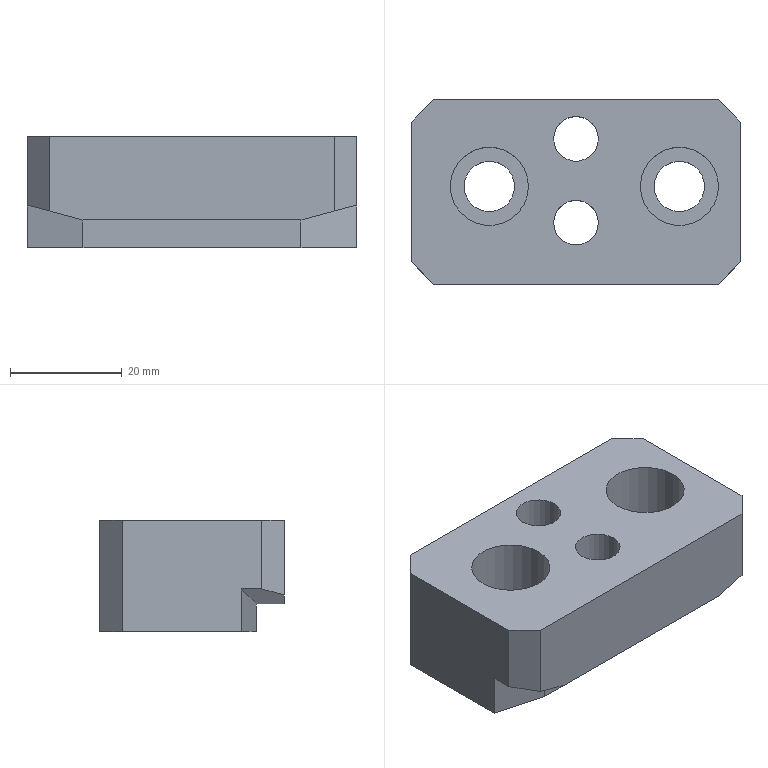Part | NX | features 20 2 | 1 solid | 24 faces | box 59 x 33 x 20 mm | volume 30264 mm3 | plane 18 | cylinder 6 | commonest cylinder face diameters 8.001 x2 9 x2 14 x2
STEP:
#1=CARTESIAN_POINT('',(2760.502,417.5,1.5));
#2=VERTEX_POINT('',#1);
#3=CARTESIAN_POINT('',(2799.502,417.5,1.5));
#4=VERTEX_POINT('',#3);
#5=CARTESIAN_POINT('',(2886.502,417.5,1.5));
#6=DIRECTION('',(1.,0.,0.));
#7=VECTOR('',#6,1000.);
#8=LINE('',#5,#7);
#9=EDGE_CURVE('',#2,#4,#8,.T.);
#10=ORIENTED_EDGE('',*,*,#9,.T.);
#11=CARTESIAN_POINT('',(2805.502,417.5,3.108));
#12=VERTEX_POINT('',#11);
#13=CARTESIAN_POINT('',(2799.502,417.5,1.5));
#14=DIRECTION('',(-0.9659,0.,-0.2588));
#15=VECTOR('',#14,1000.);
#16=LINE('',#13,#15);
#17=EDGE_CURVE('',#12,#4,#16,.T.);
#18=ORIENTED_EDGE('',*,*,#17,.F.);
#19=CARTESIAN_POINT('',(2805.502,417.5,16.5));
#20=VERTEX_POINT('',#19);
#21=CARTESIAN_POINT('',(2805.502,417.5,11.5));
#22=DIRECTION('',(0.,0.,-1.));
#23=VECTOR('',#22,1000.);
#24=LINE('',#21,#23);
#25=EDGE_CURVE('',#20,#12,#24,.T.);
#26=ORIENTED_EDGE('',*,*,#25,.F.);
#27=CARTESIAN_POINT('',(2754.502,417.5,16.5));
#28=VERTEX_POINT('',#27);
#29=CARTESIAN_POINT('',(2908.502,417.5,16.5));
#30=DIRECTION('',(-1.,0.,0.));
#31=VECTOR('',#30,1000.);
#32=LINE('',#29,#31);
#33=EDGE_CURVE('',#20,#28,#32,.T.);
#34=ORIENTED_EDGE('',*,*,#33,.T.);
#35=CARTESIAN_POINT('',(2754.502,417.5,3.108));
#36=VERTEX_POINT('',#35);
#37=CARTESIAN_POINT('',(2754.502,417.5,11.5));
#38=DIRECTION('',(0.,0.,1.));
#39=VECTOR('',#38,1000.);
#40=LINE('',#37,#39);
#41=EDGE_CURVE('',#36,#28,#40,.T.);
#42=ORIENTED_EDGE('',*,*,#41,.F.);
#43=CARTESIAN_POINT('',(2760.502,417.5,1.5));
#44=DIRECTION('',(-0.9659,0.,0.2588));
#45=VECTOR('',#44,1000.);
#46=LINE('',#43,#45);
#47=EDGE_CURVE('',#2,#36,#46,.T.);
#48=ORIENTED_EDGE('',*,*,#47,.F.);
#49=EDGE_LOOP('',(#10,#18,#26,#34,#42,#48));
#50=FACE_BOUND('',#49,.T.);
#51=CARTESIAN_POINT('',(2908.502,417.5,11.5));
#52=DIRECTION('',(0.,1.,0.));
#53=DIRECTION('',(0.,0.,1.));
#54=AXIS2_PLACEMENT_3D('',#51,#52,#53);
#55=PLANE('',#54);
#56=ADVANCED_FACE('',(#50),#55,.F.);
#57=CARTESIAN_POINT('',(2784.003,428.5,16.5));
#58=VERTEX_POINT('',#57);
#59=CARTESIAN_POINT('',(2780.002,428.5,16.5));
#60=DIRECTION('',(0.,0.,1.));
#61=DIRECTION('',(1.,0.,0.));
#62=AXIS2_PLACEMENT_3D('',#59,#60,#61);
#63=CIRCLE('',#62,4.);
#64=EDGE_CURVE('',#58,#58,#63,.T.);
#65=ORIENTED_EDGE('',*,*,#64,.F.);
#66=EDGE_LOOP('',(#65));
#67=FACE_BOUND('',#66,.T.);
#68=CARTESIAN_POINT('',(2784.003,443.5,16.5));
#69=VERTEX_POINT('',#68);
#70=CARTESIAN_POINT('',(2780.002,443.5,16.5));
#71=DIRECTION('',(0.,0.,1.));
#72=DIRECTION('',(1.,0.,0.));
#73=AXIS2_PLACEMENT_3D('',#70,#71,#72);
#74=CIRCLE('',#73,4.);
#75=EDGE_CURVE('',#69,#69,#74,.T.);
#76=ORIENTED_EDGE('',*,*,#75,.F.);
#77=EDGE_LOOP('',(#76));
#78=FACE_BOUND('',#77,.T.);
#79=CARTESIAN_POINT('',(2805.502,435.,16.5));
#80=VERTEX_POINT('',#79);
#81=CARTESIAN_POINT('',(2798.502,435.,16.5));
#82=DIRECTION('',(0.,0.,-1.));
#83=DIRECTION('',(1.,0.,0.));
#84=AXIS2_PLACEMENT_3D('',#81,#82,#83);
#85=CIRCLE('',#84,7.);
#86=EDGE_CURVE('',#80,#80,#85,.T.);
#87=ORIENTED_EDGE('',*,*,#86,.T.);
#88=EDGE_LOOP('',(#87));
#89=FACE_BOUND('',#88,.T.);
#90=CARTESIAN_POINT('',(2771.502,435.,16.5));
#91=VERTEX_POINT('',#90);
#92=CARTESIAN_POINT('',(2764.502,435.,16.5));
#93=DIRECTION('',(0.,0.,-1.));
#94=DIRECTION('',(1.,0.,0.));
#95=AXIS2_PLACEMENT_3D('',#92,#93,#94);
#96=CIRCLE('',#95,7.);
#97=EDGE_CURVE('',#91,#91,#96,.T.);
#98=ORIENTED_EDGE('',*,*,#97,.T.);
#99=EDGE_LOOP('',(#98));
#100=FACE_BOUND('',#99,.T.);
#101=ORIENTED_EDGE('',*,*,#33,.F.);
#102=CARTESIAN_POINT('',(2809.502,421.5,16.5));
#103=VERTEX_POINT('',#102);
#104=CARTESIAN_POINT('',(2805.502,417.5,16.5));
#105=DIRECTION('',(-0.7071,-0.7071,0.));
#106=VECTOR('',#105,1000.);
#107=LINE('',#104,#106);
#108=EDGE_CURVE('',#103,#20,#107,.T.);
#109=ORIENTED_EDGE('',*,*,#108,.F.);
#110=CARTESIAN_POINT('',(2809.502,446.5,16.5));
#111=VERTEX_POINT('',#110);
#112=CARTESIAN_POINT('',(2809.502,450.5,16.5));
#113=DIRECTION('',(0.,-1.,0.));
#114=VECTOR('',#113,1000.);
#115=LINE('',#112,#114);
#116=EDGE_CURVE('',#111,#103,#115,.T.);
#117=ORIENTED_EDGE('',*,*,#116,.F.);
#118=CARTESIAN_POINT('',(2805.502,450.5,16.5));
#119=VERTEX_POINT('',#118);
#120=CARTESIAN_POINT('',(2809.502,446.5,16.5));
#121=DIRECTION('',(0.7071,-0.7071,0.));
#122=VECTOR('',#121,1000.);
#123=LINE('',#120,#122);
#124=EDGE_CURVE('',#119,#111,#123,.T.);
#125=ORIENTED_EDGE('',*,*,#124,.F.);
#126=CARTESIAN_POINT('',(2754.502,450.5,16.5));
#127=VERTEX_POINT('',#126);
#128=CARTESIAN_POINT('',(2828.502,450.5,16.5));
#129=DIRECTION('',(1.,0.,0.));
#130=VECTOR('',#129,1000.);
#131=LINE('',#128,#130);
#132=EDGE_CURVE('',#127,#119,#131,.T.);
#133=ORIENTED_EDGE('',*,*,#132,.F.);
#134=CARTESIAN_POINT('',(2750.502,446.5,16.5));
#135=VERTEX_POINT('',#134);
#136=CARTESIAN_POINT('',(2754.502,450.5,16.5));
#137=DIRECTION('',(0.7071,0.7071,0.));
#138=VECTOR('',#137,1000.);
#139=LINE('',#136,#138);
#140=EDGE_CURVE('',#135,#127,#139,.T.);
#141=ORIENTED_EDGE('',*,*,#140,.F.);
#142=CARTESIAN_POINT('',(2750.502,421.5,16.5));
#143=VERTEX_POINT('',#142);
#144=CARTESIAN_POINT('',(2750.502,417.5,16.5));
#145=DIRECTION('',(0.,1.,0.));
#146=VECTOR('',#145,1000.);
#147=LINE('',#144,#146);
#148=EDGE_CURVE('',#143,#135,#147,.T.);
#149=ORIENTED_EDGE('',*,*,#148,.F.);
#150=CARTESIAN_POINT('',(2750.502,421.5,16.5));
#151=DIRECTION('',(-0.7071,0.7071,0.));
#152=VECTOR('',#151,1000.);
#153=LINE('',#150,#152);
#154=EDGE_CURVE('',#28,#143,#153,.T.);
#155=ORIENTED_EDGE('',*,*,#154,.F.);
#156=EDGE_LOOP('',(#101,#109,#117,#125,#133,#141,#149,#155));
#157=FACE_BOUND('',#156,.T.);
#158=CARTESIAN_POINT('',(2908.502,450.5,16.5));
#159=DIRECTION('',(0.,0.,1.));
#160=DIRECTION('',(-1.,0.,0.));
#161=AXIS2_PLACEMENT_3D('',#158,#159,#160);
#162=PLANE('',#161);
#163=ADVANCED_FACE('',(#67,#78,#89,#100,#157),#162,.T.);
#164=CARTESIAN_POINT('',(2794.002,435.,6.5));
#165=VERTEX_POINT('',#164);
#166=CARTESIAN_POINT('',(2798.502,435.,6.5));
#167=DIRECTION('',(0.,0.,1.));
#168=DIRECTION('',(-1.,0.,0.));
#169=AXIS2_PLACEMENT_3D('',#166,#167,#168);
#170=CIRCLE('',#169,4.5);
#171=EDGE_CURVE('',#165,#165,#170,.T.);
#172=ORIENTED_EDGE('',*,*,#171,.F.);
#173=EDGE_LOOP('',(#172));
#174=FACE_BOUND('',#173,.T.);
#175=CARTESIAN_POINT('',(2791.502,435.,6.5));
#176=VERTEX_POINT('',#175);
#177=CARTESIAN_POINT('',(2798.502,435.,6.5));
#178=DIRECTION('',(0.,0.,-1.));
#179=DIRECTION('',(-1.,0.,0.));
#180=AXIS2_PLACEMENT_3D('',#177,#178,#179);
#181=CIRCLE('',#180,7.);
#182=EDGE_CURVE('',#176,#176,#181,.T.);
#183=ORIENTED_EDGE('',*,*,#182,.F.);
#184=EDGE_LOOP('',(#183));
#185=FACE_BOUND('',#184,.T.);
#186=CARTESIAN_POINT('',(2798.502,432.5,6.5));
#187=DIRECTION('',(0.,0.,-1.));
#188=DIRECTION('',(1.,0.,0.));
#189=AXIS2_PLACEMENT_3D('',#186,#187,#188);
#190=PLANE('',#189);
#191=ADVANCED_FACE('',(#174,#185),#190,.F.);
#192=CARTESIAN_POINT('',(2799.502,422.5,1.5));
#193=VERTEX_POINT('',#192);
#194=CARTESIAN_POINT('',(2799.502,425.18,1.5));
#195=DIRECTION('',(0.,1.,0.));
#196=VECTOR('',#195,1000.);
#197=LINE('',#194,#196);
#198=EDGE_CURVE('',#4,#193,#197,.T.);
#199=ORIENTED_EDGE('',*,*,#198,.T.);
#200=CARTESIAN_POINT('',(2809.502,425.18,4.179));
#201=VERTEX_POINT('',#200);
#202=CARTESIAN_POINT('',(2808.875,425.012,4.011));
#203=DIRECTION('',(0.9351,0.2506,0.2506));
#204=VECTOR('',#203,1000.);
#205=LINE('',#202,#204);
#206=EDGE_CURVE('',#193,#201,#205,.T.);
#207=ORIENTED_EDGE('',*,*,#206,.T.);
#208=CARTESIAN_POINT('',(2809.502,421.5,4.179));
#209=VERTEX_POINT('',#208);
#210=CARTESIAN_POINT('',(2809.502,417.5,4.179));
#211=DIRECTION('',(0.,-1.,0.));
#212=VECTOR('',#211,1000.);
#213=LINE('',#210,#212);
#214=EDGE_CURVE('',#201,#209,#213,.T.);
#215=ORIENTED_EDGE('',*,*,#214,.T.);
#216=CARTESIAN_POINT('',(2792.451,404.449,-0.3894));
#217=DIRECTION('',(0.6947,0.6947,0.1862));
#218=VECTOR('',#217,1000.);
#219=LINE('',#216,#218);
#220=EDGE_CURVE('',#12,#209,#219,.T.);
#221=ORIENTED_EDGE('',*,*,#220,.F.);
#222=ORIENTED_EDGE('',*,*,#17,.T.);
#223=EDGE_LOOP('',(#199,#207,#215,#221,#222));
#224=FACE_BOUND('',#223,.T.);
#225=CARTESIAN_POINT('',(2799.502,396.891,1.5));
#226=DIRECTION('',(0.2588,0.,-0.9659));
#227=DIRECTION('',(0.9659,0.,0.2588));
#228=AXIS2_PLACEMENT_3D('',#225,#226,#227);
#229=PLANE('',#228);
#230=ADVANCED_FACE('',(#224),#229,.T.);
#231=CARTESIAN_POINT('',(2760.002,435.,6.5));
#232=VERTEX_POINT('',#231);
#233=CARTESIAN_POINT('',(2764.502,435.,6.5));
#234=DIRECTION('',(0.,0.,1.));
#235=DIRECTION('',(-1.,0.,0.));
#236=AXIS2_PLACEMENT_3D('',#233,#234,#235);
#237=CIRCLE('',#236,4.5);
#238=EDGE_CURVE('',#232,#232,#237,.T.);
#239=ORIENTED_EDGE('',*,*,#238,.F.);
#240=EDGE_LOOP('',(#239));
#241=FACE_BOUND('',#240,.T.);
#242=CARTESIAN_POINT('',(2757.502,435.,6.5));
#243=VERTEX_POINT('',#242);
#244=CARTESIAN_POINT('',(2764.502,435.,6.5));
#245=DIRECTION('',(0.,0.,-1.));
#246=DIRECTION('',(-1.,0.,0.));
#247=AXIS2_PLACEMENT_3D('',#244,#245,#246);
#248=CIRCLE('',#247,7.);
#249=EDGE_CURVE('',#243,#243,#248,.T.);
#250=ORIENTED_EDGE('',*,*,#249,.F.);
#251=EDGE_LOOP('',(#250));
#252=FACE_BOUND('',#251,.T.);
#253=CARTESIAN_POINT('',(2764.502,432.5,6.5));
#254=DIRECTION('',(0.,0.,-1.));
#255=DIRECTION('',(-1.,0.,0.));
#256=AXIS2_PLACEMENT_3D('',#253,#254,#255);
#257=PLANE('',#256);
#258=ADVANCED_FACE('',(#241,#252),#257,.F.);
#259=ORIENTED_EDGE('',*,*,#86,.F.);
#260=EDGE_LOOP('',(#259));
#261=FACE_BOUND('',#260,.T.);
#262=ORIENTED_EDGE('',*,*,#182,.T.);
#263=EDGE_LOOP('',(#262));
#264=FACE_BOUND('',#263,.T.);
#265=CARTESIAN_POINT('',(2798.502,435.,42.5));
#266=DIRECTION('',(0.,0.,-1.));
#267=DIRECTION('',(1.,0.,0.));
#268=AXIS2_PLACEMENT_3D('',#265,#266,#267);
#269=CYLINDRICAL_SURFACE('',#268,7.);
#270=ADVANCED_FACE('',(#261,#264),#269,.F.);
#271=ORIENTED_EDGE('',*,*,#108,.T.);
#272=ORIENTED_EDGE('',*,*,#25,.T.);
#273=ORIENTED_EDGE('',*,*,#220,.T.);
#274=CARTESIAN_POINT('',(2809.502,421.5,11.5));
#275=DIRECTION('',(0.,0.,1.));
#276=VECTOR('',#275,1000.);
#277=LINE('',#274,#276);
#278=EDGE_CURVE('',#209,#103,#277,.T.);
#279=ORIENTED_EDGE('',*,*,#278,.T.);
#280=EDGE_LOOP('',(#271,#272,#273,#279));
#281=FACE_BOUND('',#280,.T.);
#282=CARTESIAN_POINT('',(2805.502,417.5,11.5));
#283=DIRECTION('',(-0.7071,0.7071,0.));
#284=DIRECTION('',(0.,0.,-1.));
#285=AXIS2_PLACEMENT_3D('',#282,#283,#284);
#286=PLANE('',#285);
#287=ADVANCED_FACE('',(#281),#286,.F.);
#288=ORIENTED_EDGE('',*,*,#249,.T.);
#289=EDGE_LOOP('',(#288));
#290=FACE_BOUND('',#289,.T.);
#291=ORIENTED_EDGE('',*,*,#97,.F.);
#292=EDGE_LOOP('',(#291));
#293=FACE_BOUND('',#292,.T.);
#294=CARTESIAN_POINT('',(2764.502,435.,42.5));
#295=DIRECTION('',(0.,0.,-1.));
#296=DIRECTION('',(-1.,0.,0.));
#297=AXIS2_PLACEMENT_3D('',#294,#295,#296);
#298=CYLINDRICAL_SURFACE('',#297,7.);
#299=ADVANCED_FACE('',(#290,#293),#298,.F.);
#300=ORIENTED_EDGE('',*,*,#214,.F.);
#301=CARTESIAN_POINT('',(2809.502,425.18,-3.5));
#302=VERTEX_POINT('',#301);
#303=CARTESIAN_POINT('',(2809.502,425.18,3.5));
#304=DIRECTION('',(0.,0.,-1.));
#305=VECTOR('',#304,1000.);
#306=LINE('',#303,#305);
#307=EDGE_CURVE('',#201,#302,#306,.T.);
#308=ORIENTED_EDGE('',*,*,#307,.T.);
#309=CARTESIAN_POINT('',(2809.502,446.5,-3.5));
#310=VERTEX_POINT('',#309);
#311=CARTESIAN_POINT('',(2809.502,450.5,-3.5));
#312=DIRECTION('',(0.,-1.,0.));
#313=VECTOR('',#312,1000.);
#314=LINE('',#311,#313);
#315=EDGE_CURVE('',#310,#302,#314,.T.);
#316=ORIENTED_EDGE('',*,*,#315,.F.);
#317=CARTESIAN_POINT('',(2809.502,446.5,11.5));
#318=DIRECTION('',(0.,0.,-1.));
#319=VECTOR('',#318,1000.);
#320=LINE('',#317,#319);
#321=EDGE_CURVE('',#111,#310,#320,.T.);
#322=ORIENTED_EDGE('',*,*,#321,.F.);
#323=ORIENTED_EDGE('',*,*,#116,.T.);
#324=ORIENTED_EDGE('',*,*,#278,.F.);
#325=EDGE_LOOP('',(#300,#308,#316,#322,#323,#324));
#326=FACE_BOUND('',#325,.T.);
#327=CARTESIAN_POINT('',(2809.502,450.5,11.5));
#328=DIRECTION('',(-1.,0.,0.));
#329=DIRECTION('',(0.,0.,-1.));
#330=AXIS2_PLACEMENT_3D('',#327,#328,#329);
#331=PLANE('',#330);
#332=ADVANCED_FACE('',(#326),#331,.F.);
#333=CARTESIAN_POINT('',(2799.501,422.5,1.5));
#334=VERTEX_POINT('',#333);
#335=CARTESIAN_POINT('',(2809.502,425.18,1.5));
#336=DIRECTION('',(0.9659,0.2588,0.));
#337=VECTOR('',#336,1000.);
#338=LINE('',#335,#337);
#339=EDGE_CURVE('',#334,#193,#338,.T.);
#340=ORIENTED_EDGE('',*,*,#339,.F.);
#341=CARTESIAN_POINT('',(2799.501,422.5,-3.5));
#342=VERTEX_POINT('',#341);
#343=CARTESIAN_POINT('',(2799.501,422.5,3.5));
#344=DIRECTION('',(0.,0.,1.));
#345=VECTOR('',#344,1000.);
#346=LINE('',#343,#345);
#347=EDGE_CURVE('',#342,#334,#346,.T.);
#348=ORIENTED_EDGE('',*,*,#347,.F.);
#349=CARTESIAN_POINT('',(2809.502,425.18,-3.5));
#350=DIRECTION('',(-0.9659,-0.2588,0.));
#351=VECTOR('',#350,1000.);
#352=LINE('',#349,#351);
#353=EDGE_CURVE('',#302,#342,#352,.T.);
#354=ORIENTED_EDGE('',*,*,#353,.F.);
#355=ORIENTED_EDGE('',*,*,#307,.F.);
#356=ORIENTED_EDGE('',*,*,#206,.F.);
#357=EDGE_LOOP('',(#340,#348,#354,#355,#356));
#358=FACE_BOUND('',#357,.T.);
#359=CARTESIAN_POINT('',(2809.502,425.18,3.5));
#360=DIRECTION('',(-0.2588,0.9659,0.));
#361=DIRECTION('',(0.9659,0.2588,0.));
#362=AXIS2_PLACEMENT_3D('',#359,#360,#361);
#363=PLANE('',#362);
#364=ADVANCED_FACE('',(#358),#363,.F.);
#365=ORIENTED_EDGE('',*,*,#171,.T.);
#366=EDGE_LOOP('',(#365));
#367=FACE_BOUND('',#366,.T.);
#368=CARTESIAN_POINT('',(2803.002,435.,-3.5));
#369=VERTEX_POINT('',#368);
#370=CARTESIAN_POINT('',(2798.502,435.,-3.5));
#371=DIRECTION('',(0.,0.,-1.));
#372=DIRECTION('',(1.,0.,0.));
#373=AXIS2_PLACEMENT_3D('',#370,#371,#372);
#374=CIRCLE('',#373,4.5);
#375=EDGE_CURVE('',#369,#369,#374,.T.);
#376=ORIENTED_EDGE('',*,*,#375,.T.);
#377=EDGE_LOOP('',(#376));
#378=FACE_BOUND('',#377,.T.);
#379=CARTESIAN_POINT('',(2798.502,435.,42.5));
#380=DIRECTION('',(0.,0.,-1.));
#381=DIRECTION('',(1.,0.,0.));
#382=AXIS2_PLACEMENT_3D('',#379,#380,#381);
#383=CYLINDRICAL_SURFACE('',#382,4.5);
#384=ADVANCED_FACE('',(#367,#378),#383,.F.);
#385=CARTESIAN_POINT('',(2750.502,421.5,4.179));
#386=VERTEX_POINT('',#385);
#387=CARTESIAN_POINT('',(2750.502,421.5,11.5));
#388=DIRECTION('',(0.,0.,-1.));
#389=VECTOR('',#388,1000.);
#390=LINE('',#387,#389);
#391=EDGE_CURVE('',#143,#386,#390,.T.);
#392=ORIENTED_EDGE('',*,*,#391,.T.);
#393=CARTESIAN_POINT('',(2767.554,404.449,-0.3894));
#394=DIRECTION('',(0.6947,-0.6947,-0.1862));
#395=VECTOR('',#394,1000.);
#396=LINE('',#393,#395);
#397=EDGE_CURVE('',#386,#36,#396,.T.);
#398=ORIENTED_EDGE('',*,*,#397,.T.);
#399=ORIENTED_EDGE('',*,*,#41,.T.);
#400=ORIENTED_EDGE('',*,*,#154,.T.);
#401=EDGE_LOOP('',(#392,#398,#399,#400));
#402=FACE_BOUND('',#401,.T.);
#403=CARTESIAN_POINT('',(2750.502,421.5,11.5));
#404=DIRECTION('',(0.7071,0.7071,0.));
#405=DIRECTION('',(0.,0.,-1.));
#406=AXIS2_PLACEMENT_3D('',#403,#404,#405);
#407=PLANE('',#406);
#408=ADVANCED_FACE('',(#402),#407,.F.);
#409=CARTESIAN_POINT('',(2769.002,435.,-3.5));
#410=VERTEX_POINT('',#409);
#411=CARTESIAN_POINT('',(2764.502,435.,-3.5));
#412=DIRECTION('',(0.,0.,1.));
#413=DIRECTION('',(1.,0.,0.));
#414=AXIS2_PLACEMENT_3D('',#411,#412,#413);
#415=CIRCLE('',#414,4.5);
#416=EDGE_CURVE('',#410,#410,#415,.T.);
#417=ORIENTED_EDGE('',*,*,#416,.F.);
#418=EDGE_LOOP('',(#417));
#419=FACE_BOUND('',#418,.T.);
#420=ORIENTED_EDGE('',*,*,#238,.T.);
#421=EDGE_LOOP('',(#420));
#422=FACE_BOUND('',#421,.T.);
#423=CARTESIAN_POINT('',(2764.502,435.,42.5));
#424=DIRECTION('',(0.,0.,-1.));
#425=DIRECTION('',(-1.,0.,0.));
#426=AXIS2_PLACEMENT_3D('',#423,#424,#425);
#427=CYLINDRICAL_SURFACE('',#426,4.5);
#428=ADVANCED_FACE('',(#419,#422),#427,.F.);
#429=CARTESIAN_POINT('',(2750.502,425.179,-3.5));
#430=VERTEX_POINT('',#429);
#431=CARTESIAN_POINT('',(2750.502,446.5,-3.5));
#432=VERTEX_POINT('',#431);
#433=CARTESIAN_POINT('',(2750.502,417.5,-3.5));
#434=DIRECTION('',(0.,1.,0.));
#435=VECTOR('',#434,1000.);
#436=LINE('',#433,#435);
#437=EDGE_CURVE('',#430,#432,#436,.T.);
#438=ORIENTED_EDGE('',*,*,#437,.F.);
#439=CARTESIAN_POINT('',(2750.502,425.179,4.179));
#440=VERTEX_POINT('',#439);
#441=CARTESIAN_POINT('',(2750.502,425.179,3.5));
#442=DIRECTION('',(0.,0.,-1.));
#443=VECTOR('',#442,1000.);
#444=LINE('',#441,#443);
#445=EDGE_CURVE('',#440,#430,#444,.T.);
#446=ORIENTED_EDGE('',*,*,#445,.F.);
#447=CARTESIAN_POINT('',(2750.502,425.179,4.179));
#448=DIRECTION('',(0.,1.,0.));
#449=VECTOR('',#448,1000.);
#450=LINE('',#447,#449);
#451=EDGE_CURVE('',#386,#440,#450,.T.);
#452=ORIENTED_EDGE('',*,*,#451,.F.);
#453=ORIENTED_EDGE('',*,*,#391,.F.);
#454=ORIENTED_EDGE('',*,*,#148,.T.);
#455=CARTESIAN_POINT('',(2750.502,446.5,11.5));
#456=DIRECTION('',(0.,0.,1.));
#457=VECTOR('',#456,1000.);
#458=LINE('',#455,#457);
#459=EDGE_CURVE('',#432,#135,#458,.T.);
#460=ORIENTED_EDGE('',*,*,#459,.F.);
#461=EDGE_LOOP('',(#438,#446,#452,#453,#454,#460));
#462=FACE_BOUND('',#461,.T.);
#463=CARTESIAN_POINT('',(2750.502,417.5,11.5));
#464=DIRECTION('',(1.,0.,0.));
#465=DIRECTION('',(0.,0.,1.));
#466=AXIS2_PLACEMENT_3D('',#463,#464,#465);
#467=PLANE('',#466);
#468=ADVANCED_FACE('',(#462),#467,.F.);
#469=ORIENTED_EDGE('',*,*,#451,.T.);
#470=CARTESIAN_POINT('',(2760.501,422.5,1.5));
#471=VERTEX_POINT('',#470);
#472=CARTESIAN_POINT('',(2760.501,422.5,1.5));
#473=DIRECTION('',(0.9351,-0.2506,-0.2506));
#474=VECTOR('',#473,1000.);
#475=LINE('',#472,#474);
#476=EDGE_CURVE('',#440,#471,#475,.T.);
#477=ORIENTED_EDGE('',*,*,#476,.T.);
#478=CARTESIAN_POINT('',(2760.502,422.5,1.5));
#479=VERTEX_POINT('',#478);
#480=CARTESIAN_POINT('',(2760.502,422.5,1.5));
#481=DIRECTION('',(0.9659,0.,-0.2588));
#482=VECTOR('',#481,1000.);
#483=LINE('',#480,#482);
#484=EDGE_CURVE('',#471,#479,#483,.T.);
#485=ORIENTED_EDGE('',*,*,#484,.T.);
#486=CARTESIAN_POINT('',(2760.502,417.5,1.5));
#487=DIRECTION('',(0.,-1.,0.));
#488=VECTOR('',#487,1000.);
#489=LINE('',#486,#488);
#490=EDGE_CURVE('',#479,#2,#489,.T.);
#491=ORIENTED_EDGE('',*,*,#490,.T.);
#492=ORIENTED_EDGE('',*,*,#47,.T.);
#493=ORIENTED_EDGE('',*,*,#397,.F.);
#494=EDGE_LOOP('',(#469,#477,#485,#491,#492,#493));
#495=FACE_BOUND('',#494,.T.);
#496=CARTESIAN_POINT('',(2760.502,396.891,1.5));
#497=DIRECTION('',(-0.2588,0.,-0.9659));
#498=DIRECTION('',(0.9659,0.,-0.2588));
#499=AXIS2_PLACEMENT_3D('',#496,#497,#498);
#500=PLANE('',#499);
#501=ADVANCED_FACE('',(#495),#500,.T.);
#502=CARTESIAN_POINT('',(2760.501,422.5,-3.5));
#503=VERTEX_POINT('',#502);
#504=CARTESIAN_POINT('',(2760.501,422.5,-3.5));
#505=DIRECTION('',(-0.9659,0.2588,0.));
#506=VECTOR('',#505,1000.);
#507=LINE('',#504,#506);
#508=EDGE_CURVE('',#503,#430,#507,.T.);
#509=ORIENTED_EDGE('',*,*,#508,.F.);
#510=CARTESIAN_POINT('',(2760.501,422.5,3.5));
#511=DIRECTION('',(0.,0.,1.));
#512=VECTOR('',#511,1000.);
#513=LINE('',#510,#512);
#514=EDGE_CURVE('',#503,#471,#513,.T.);
#515=ORIENTED_EDGE('',*,*,#514,.T.);
#516=ORIENTED_EDGE('',*,*,#476,.F.);
#517=ORIENTED_EDGE('',*,*,#445,.T.);
#518=EDGE_LOOP('',(#509,#515,#516,#517));
#519=FACE_BOUND('',#518,.T.);
#520=CARTESIAN_POINT('',(2760.501,422.5,3.5));
#521=DIRECTION('',(0.2588,0.9659,0.));
#522=DIRECTION('',(0.9659,-0.2588,0.));
#523=AXIS2_PLACEMENT_3D('',#520,#521,#522);
#524=PLANE('',#523);
#525=ADVANCED_FACE('',(#519),#524,.F.);
#526=CARTESIAN_POINT('',(2784.003,428.5,-3.5));
#527=VERTEX_POINT('',#526);
#528=CARTESIAN_POINT('',(2780.002,428.5,-3.5));
#529=DIRECTION('',(0.,0.,1.));
#530=DIRECTION('',(1.,0.,0.));
#531=AXIS2_PLACEMENT_3D('',#528,#529,#530);
#532=CIRCLE('',#531,4.);
#533=EDGE_CURVE('',#527,#527,#532,.T.);
#534=ORIENTED_EDGE('',*,*,#533,.T.);
#535=EDGE_LOOP('',(#534));
#536=FACE_BOUND('',#535,.T.);
#537=CARTESIAN_POINT('',(2784.003,443.5,-3.5));
#538=VERTEX_POINT('',#537);
#539=CARTESIAN_POINT('',(2780.002,443.5,-3.5));
#540=DIRECTION('',(0.,0.,1.));
#541=DIRECTION('',(1.,0.,0.));
#542=AXIS2_PLACEMENT_3D('',#539,#540,#541);
#543=CIRCLE('',#542,4.);
#544=EDGE_CURVE('',#538,#538,#543,.T.);
#545=ORIENTED_EDGE('',*,*,#544,.T.);
#546=EDGE_LOOP('',(#545));
#547=FACE_BOUND('',#546,.T.);
#548=CARTESIAN_POINT('',(2846.501,422.5,-3.5));
#549=DIRECTION('',(-1.,0.,0.));
#550=VECTOR('',#549,1000.);
#551=LINE('',#548,#550);
#552=EDGE_CURVE('',#342,#503,#551,.T.);
#553=ORIENTED_EDGE('',*,*,#552,.T.);
#554=ORIENTED_EDGE('',*,*,#508,.T.);
#555=ORIENTED_EDGE('',*,*,#437,.T.);
#556=CARTESIAN_POINT('',(2754.502,450.5,-3.5));
#557=VERTEX_POINT('',#556);
#558=CARTESIAN_POINT('',(2754.502,450.5,-3.5));
#559=DIRECTION('',(-0.7071,-0.7071,0.));
#560=VECTOR('',#559,1000.);
#561=LINE('',#558,#560);
#562=EDGE_CURVE('',#557,#432,#561,.T.);
#563=ORIENTED_EDGE('',*,*,#562,.F.);
#564=CARTESIAN_POINT('',(2805.502,450.5,-3.5));
#565=VERTEX_POINT('',#564);
#566=CARTESIAN_POINT('',(2868.502,450.5,-3.5));
#567=DIRECTION('',(1.,0.,0.));
#568=VECTOR('',#567,1000.);
#569=LINE('',#566,#568);
#570=EDGE_CURVE('',#557,#565,#569,.T.);
#571=ORIENTED_EDGE('',*,*,#570,.T.);
#572=CARTESIAN_POINT('',(2809.502,446.5,-3.5));
#573=DIRECTION('',(-0.7071,0.7071,0.));
#574=VECTOR('',#573,1000.);
#575=LINE('',#572,#574);
#576=EDGE_CURVE('',#310,#565,#575,.T.);
#577=ORIENTED_EDGE('',*,*,#576,.F.);
#578=ORIENTED_EDGE('',*,*,#315,.T.);
#579=ORIENTED_EDGE('',*,*,#353,.T.);
#580=EDGE_LOOP('',(#553,#554,#555,#563,#571,#577,#578,#579));
#581=FACE_BOUND('',#580,.T.);
#582=ORIENTED_EDGE('',*,*,#416,.T.);
#583=EDGE_LOOP('',(#582));
#584=FACE_BOUND('',#583,.T.);
#585=ORIENTED_EDGE('',*,*,#375,.F.);
#586=EDGE_LOOP('',(#585));
#587=FACE_BOUND('',#586,.T.);
#588=CARTESIAN_POINT('',(2938.502,450.5,-3.5));
#589=DIRECTION('',(0.,0.,1.));
#590=DIRECTION('',(-1.,0.,0.));
#591=AXIS2_PLACEMENT_3D('',#588,#589,#590);
#592=PLANE('',#591);
#593=ADVANCED_FACE('',(#536,#547,#581,#584,#587),#592,.F.);
#594=ORIENTED_EDGE('',*,*,#562,.T.);
#595=ORIENTED_EDGE('',*,*,#459,.T.);
#596=ORIENTED_EDGE('',*,*,#140,.T.);
#597=CARTESIAN_POINT('',(2754.502,450.5,11.5));
#598=DIRECTION('',(0.,0.,-1.));
#599=VECTOR('',#598,1000.);
#600=LINE('',#597,#599);
#601=EDGE_CURVE('',#127,#557,#600,.T.);
#602=ORIENTED_EDGE('',*,*,#601,.T.);
#603=EDGE_LOOP('',(#594,#595,#596,#602));
#604=FACE_BOUND('',#603,.T.);
#605=CARTESIAN_POINT('',(2754.502,450.5,11.5));
#606=DIRECTION('',(0.7071,-0.7071,0.));
#607=DIRECTION('',(0.,0.,-1.));
#608=AXIS2_PLACEMENT_3D('',#605,#606,#607);
#609=PLANE('',#608);
#610=ADVANCED_FACE('',(#604),#609,.F.);
#611=ORIENTED_EDGE('',*,*,#576,.T.);
#612=CARTESIAN_POINT('',(2805.502,450.5,11.5));
#613=DIRECTION('',(0.,0.,1.));
#614=VECTOR('',#613,1000.);
#615=LINE('',#612,#614);
#616=EDGE_CURVE('',#565,#119,#615,.T.);
#617=ORIENTED_EDGE('',*,*,#616,.T.);
#618=ORIENTED_EDGE('',*,*,#124,.T.);
#619=ORIENTED_EDGE('',*,*,#321,.T.);
#620=EDGE_LOOP('',(#611,#617,#618,#619));
#621=FACE_BOUND('',#620,.T.);
#622=CARTESIAN_POINT('',(2809.502,446.5,11.5));
#623=DIRECTION('',(-0.7071,-0.7071,0.));
#624=DIRECTION('',(0.,0.,-1.));
#625=AXIS2_PLACEMENT_3D('',#622,#623,#624);
#626=PLANE('',#625);
#627=ADVANCED_FACE('',(#621),#626,.F.);
#628=ORIENTED_EDGE('',*,*,#616,.F.);
#629=ORIENTED_EDGE('',*,*,#570,.F.);
#630=ORIENTED_EDGE('',*,*,#601,.F.);
#631=ORIENTED_EDGE('',*,*,#132,.T.);
#632=EDGE_LOOP('',(#628,#629,#630,#631));
#633=FACE_BOUND('',#632,.T.);
#634=CARTESIAN_POINT('',(2828.502,450.5,11.5));
#635=DIRECTION('',(0.,-1.,0.));
#636=DIRECTION('',(0.,0.,-1.));
#637=AXIS2_PLACEMENT_3D('',#634,#635,#636);
#638=PLANE('',#637);
#639=ADVANCED_FACE('',(#633),#638,.F.);
#640=CARTESIAN_POINT('',(2876.501,422.5,1.5));
#641=DIRECTION('',(1.,0.,0.));
#642=VECTOR('',#641,1000.);
#643=LINE('',#640,#642);
#644=EDGE_CURVE('',#479,#334,#643,.T.);
#645=ORIENTED_EDGE('',*,*,#644,.T.);
#646=ORIENTED_EDGE('',*,*,#339,.T.);
#647=ORIENTED_EDGE('',*,*,#198,.F.);
#648=ORIENTED_EDGE('',*,*,#9,.F.);
#649=ORIENTED_EDGE('',*,*,#490,.F.);
#650=EDGE_LOOP('',(#645,#646,#647,#648,#649));
#651=FACE_BOUND('',#650,.T.);
#652=CARTESIAN_POINT('',(2908.773,396.891,1.5));
#653=DIRECTION('',(0.,0.,-1.));
#654=DIRECTION('',(1.,0.,0.));
#655=AXIS2_PLACEMENT_3D('',#652,#653,#654);
#656=PLANE('',#655);
#657=ADVANCED_FACE('',(#651),#656,.T.);
#658=ORIENTED_EDGE('',*,*,#347,.T.);
#659=ORIENTED_EDGE('',*,*,#644,.F.);
#660=ORIENTED_EDGE('',*,*,#484,.F.);
#661=ORIENTED_EDGE('',*,*,#514,.F.);
#662=ORIENTED_EDGE('',*,*,#552,.F.);
#663=EDGE_LOOP('',(#658,#659,#660,#661,#662));
#664=FACE_BOUND('',#663,.T.);
#665=CARTESIAN_POINT('',(2846.501,422.5,3.5));
#666=DIRECTION('',(0.,1.,0.));
#667=DIRECTION('',(0.,0.,1.));
#668=AXIS2_PLACEMENT_3D('',#665,#666,#667);
#669=PLANE('',#668);
#670=ADVANCED_FACE('',(#664),#669,.F.);
#671=ORIENTED_EDGE('',*,*,#75,.T.);
#672=EDGE_LOOP('',(#671));
#673=FACE_BOUND('',#672,.T.);
#674=ORIENTED_EDGE('',*,*,#544,.F.);
#675=EDGE_LOOP('',(#674));
#676=FACE_BOUND('',#675,.T.);
#677=CARTESIAN_POINT('',(2780.002,443.5,-83.5));
#678=DIRECTION('',(0.,0.,1.));
#679=DIRECTION('',(-1.,0.,0.));
#680=AXIS2_PLACEMENT_3D('',#677,#678,#679);
#681=CYLINDRICAL_SURFACE('',#680,4.);
#682=ADVANCED_FACE('',(#673,#676),#681,.F.);
#683=ORIENTED_EDGE('',*,*,#64,.T.);
#684=EDGE_LOOP('',(#683));
#685=FACE_BOUND('',#684,.T.);
#686=ORIENTED_EDGE('',*,*,#533,.F.);
#687=EDGE_LOOP('',(#686));
#688=FACE_BOUND('',#687,.T.);
#689=CARTESIAN_POINT('',(2780.002,428.5,-83.5));
#690=DIRECTION('',(0.,0.,1.));
#691=DIRECTION('',(-1.,0.,0.));
#692=AXIS2_PLACEMENT_3D('',#689,#690,#691);
#693=CYLINDRICAL_SURFACE('',#692,4.);
#694=ADVANCED_FACE('',(#685,#688),#693,.F.);
#695=CLOSED_SHELL('',(#56,#163,#191,#230,#258,#270,#287,#299,#332,#364,#384,#408,#428,#468,#501,#525,#593,#610,#627,#639,#657,#670,#682,#694));
#696=MANIFOLD_SOLID_BREP('',#695);
#697=(LENGTH_UNIT()NAMED_UNIT(*)SI_UNIT(.MILLI.,.METRE.));
#698=UNCERTAINTY_MEASURE_WITH_UNIT(LENGTH_MEASURE(0.00001),#697,'','');
#699=(NAMED_UNIT(*)PLANE_ANGLE_UNIT()SI_UNIT($,.RADIAN.));
#700=(NAMED_UNIT(*)SI_UNIT($,.STERADIAN.)SOLID_ANGLE_UNIT());
#701=(GEOMETRIC_REPRESENTATION_CONTEXT(3)GLOBAL_UNCERTAINTY_ASSIGNED_CONTEXT((#698))GLOBAL_UNIT_ASSIGNED_CONTEXT((#697,#699,#700))REPRESENTATION_CONTEXT('',''));
#702=ADVANCED_BREP_SHAPE_REPRESENTATION('',(#696),#701);